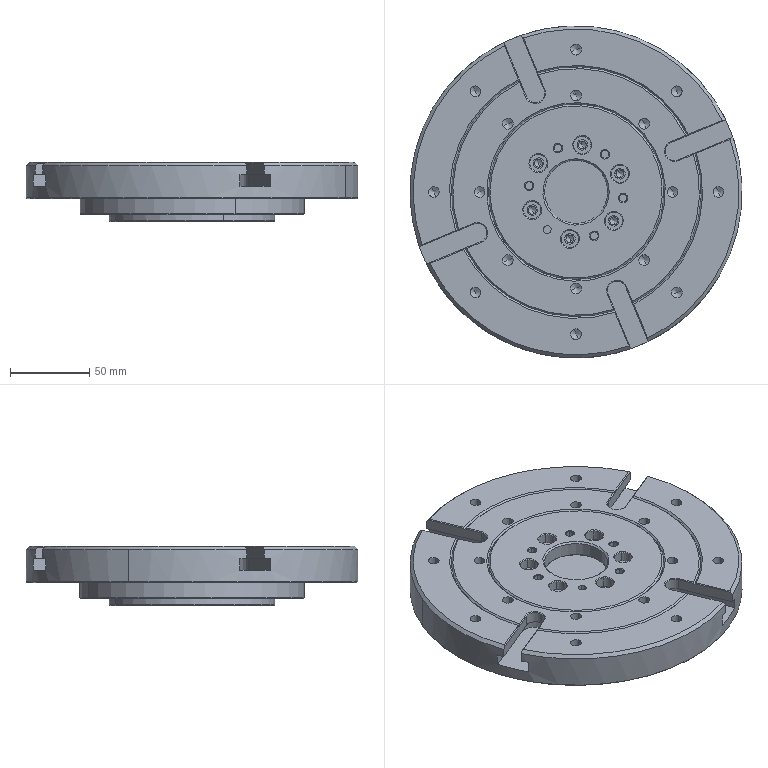NC program | Mastercam | posted with a generic post
Lines 19378 to 19401 of 19401:
(10 CHM |TOOL - 3|DIA. OFF. - 3|LEN. - 3|TOOL DIA. - 10.)
N9120 T3 M6
N9122 G0 G54 G90 X-22.175 Y18.5 C0. B180. S2000 M3
N9124 G43 H3 Z59.5
N9126 G81 G98 Z7.5 R10.5 F100.
N9128 G80
N9130 M5
N9132 G0 G28 G91 Z0.
N9134 G28 B0.
N9136 M01
N9138 G0 G17 G40 G80 G90 G94 G98
N9140 G0 G28 G91 Z0.
(8.5 DR |TOOL - 4|DIA. OFF. - 4|LEN. - 4|TOOL DIA. - 8.5)
N9142 T4 M6
N9144 G0 G54 G90 X-22.175 Y18.5 C0. B180. S1000 M3
N9146 G43 H4 Z59.5
N9148 G83 G98 Z-23.5 R10.5 Q5. F120.
N9150 G80
N9152 M5
N9154 G0 G28 G91 Z0.
N9156 G0 G28 X0. Y0.
N9158 G28 B0.
N9160 M30
%